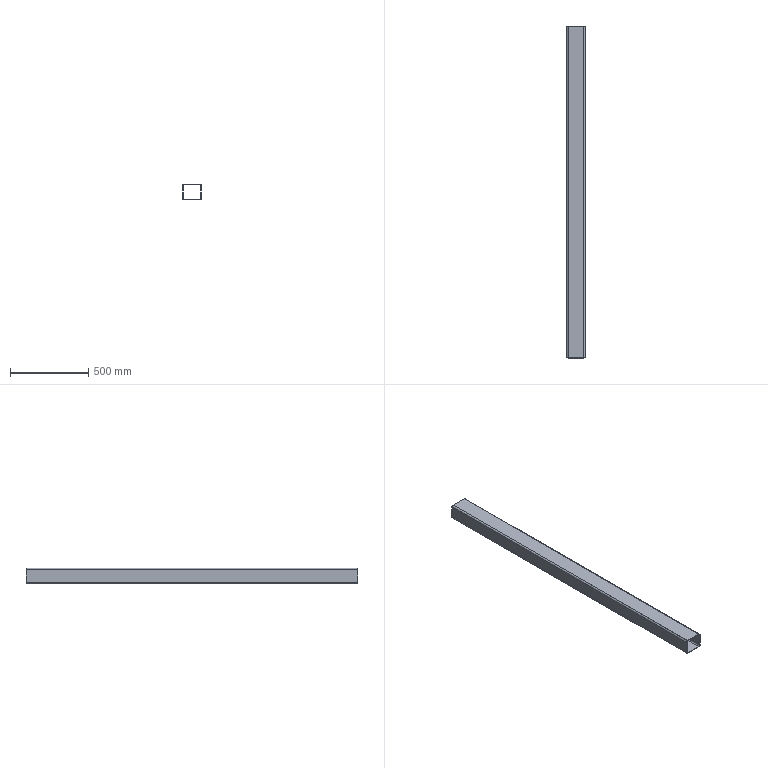Part | SolidWorks | features ExtruThin 1 | 1 solid | 18 faces | box 120 x 2124 x 100 mm | volume 2634230 mm3 | plane 10 | cylinder 8 | commonest cylinder face diameters 14 x4 20 x4
STEP:
#1=CARTESIAN_POINT('',(60.,1062.,-40.));
#2=VERTEX_POINT('',#1);
#3=CARTESIAN_POINT('',(50.,1062.,-50.));
#4=VERTEX_POINT('',#3);
#5=CARTESIAN_POINT('',(50.,1062.,-40.));
#6=DIRECTION('',(0.,1.,0.));
#7=DIRECTION('',(0.,0.,-1.));
#8=AXIS2_PLACEMENT_3D('',#5,#6,#7);
#9=CIRCLE('',#8,10.);
#10=EDGE_CURVE('',#2,#4,#9,.T.);
#11=ORIENTED_EDGE('',*,*,#10,.T.);
#12=CARTESIAN_POINT('',(-50.,1062.,-50.));
#13=VERTEX_POINT('',#12);
#14=CARTESIAN_POINT('',(-50.,1062.,-50.));
#15=DIRECTION('',(-1.,0.,0.));
#16=VECTOR('',#15,1000.);
#17=LINE('',#14,#16);
#18=EDGE_CURVE('',#4,#13,#17,.T.);
#19=ORIENTED_EDGE('',*,*,#18,.T.);
#20=CARTESIAN_POINT('',(-60.,1062.,-40.));
#21=VERTEX_POINT('',#20);
#22=CARTESIAN_POINT('',(-50.,1062.,-40.));
#23=DIRECTION('',(0.,1.,0.));
#24=DIRECTION('',(0.,0.,1.));
#25=AXIS2_PLACEMENT_3D('',#22,#23,#24);
#26=CIRCLE('',#25,10.);
#27=EDGE_CURVE('',#13,#21,#26,.T.);
#28=ORIENTED_EDGE('',*,*,#27,.T.);
#29=CARTESIAN_POINT('',(-60.,1062.,40.));
#30=VERTEX_POINT('',#29);
#31=CARTESIAN_POINT('',(-60.,1062.,-40.));
#32=DIRECTION('',(0.,0.,1.));
#33=VECTOR('',#32,1000.);
#34=LINE('',#31,#33);
#35=EDGE_CURVE('',#21,#30,#34,.T.);
#36=ORIENTED_EDGE('',*,*,#35,.T.);
#37=CARTESIAN_POINT('',(-50.,1062.,50.));
#38=VERTEX_POINT('',#37);
#39=CARTESIAN_POINT('',(-50.,1062.,40.));
#40=DIRECTION('',(0.,1.,0.));
#41=DIRECTION('',(0.,0.,1.));
#42=AXIS2_PLACEMENT_3D('',#39,#40,#41);
#43=CIRCLE('',#42,10.);
#44=EDGE_CURVE('',#30,#38,#43,.T.);
#45=ORIENTED_EDGE('',*,*,#44,.T.);
#46=CARTESIAN_POINT('',(50.,1062.,50.));
#47=VERTEX_POINT('',#46);
#48=CARTESIAN_POINT('',(-50.,1062.,50.));
#49=DIRECTION('',(1.,0.,0.));
#50=VECTOR('',#49,1000.);
#51=LINE('',#48,#50);
#52=EDGE_CURVE('',#38,#47,#51,.T.);
#53=ORIENTED_EDGE('',*,*,#52,.T.);
#54=CARTESIAN_POINT('',(60.,1062.,40.));
#55=VERTEX_POINT('',#54);
#56=CARTESIAN_POINT('',(50.,1062.,40.));
#57=DIRECTION('',(0.,1.,0.));
#58=DIRECTION('',(0.,0.,1.));
#59=AXIS2_PLACEMENT_3D('',#56,#57,#58);
#60=CIRCLE('',#59,10.);
#61=EDGE_CURVE('',#47,#55,#60,.T.);
#62=ORIENTED_EDGE('',*,*,#61,.T.);
#63=CARTESIAN_POINT('',(60.,1062.,-40.));
#64=DIRECTION('',(0.,0.,-1.));
#65=VECTOR('',#64,1000.);
#66=LINE('',#63,#65);
#67=EDGE_CURVE('',#55,#2,#66,.T.);
#68=ORIENTED_EDGE('',*,*,#67,.T.);
#69=EDGE_LOOP('',(#11,#19,#28,#36,#45,#53,#62,#68));
#70=FACE_OUTER_BOUND('',#69,.T.);
#71=CARTESIAN_POINT('',(50.,1062.,-47.));
#72=VERTEX_POINT('',#71);
#73=CARTESIAN_POINT('',(-50.,1062.,-47.));
#74=VERTEX_POINT('',#73);
#75=CARTESIAN_POINT('',(50.,1062.,-47.));
#76=DIRECTION('',(-1.,0.,0.));
#77=VECTOR('',#76,1000.);
#78=LINE('',#75,#77);
#79=EDGE_CURVE('',#72,#74,#78,.T.);
#80=ORIENTED_EDGE('',*,*,#79,.F.);
#81=CARTESIAN_POINT('',(57.,1062.,-40.));
#82=VERTEX_POINT('',#81);
#83=CARTESIAN_POINT('',(50.,1062.,-40.));
#84=DIRECTION('',(0.,1.,0.));
#85=DIRECTION('',(-1.,0.,0.));
#86=AXIS2_PLACEMENT_3D('',#83,#84,#85);
#87=CIRCLE('',#86,7.);
#88=EDGE_CURVE('',#82,#72,#87,.T.);
#89=ORIENTED_EDGE('',*,*,#88,.F.);
#90=CARTESIAN_POINT('',(57.,1062.,40.));
#91=VERTEX_POINT('',#90);
#92=CARTESIAN_POINT('',(57.,1062.,-40.));
#93=DIRECTION('',(0.,0.,-1.));
#94=VECTOR('',#93,1000.);
#95=LINE('',#92,#94);
#96=EDGE_CURVE('',#91,#82,#95,.T.);
#97=ORIENTED_EDGE('',*,*,#96,.F.);
#98=CARTESIAN_POINT('',(50.,1062.,47.));
#99=VERTEX_POINT('',#98);
#100=CARTESIAN_POINT('',(50.,1062.,40.));
#101=DIRECTION('',(0.,1.,0.));
#102=DIRECTION('',(-1.,0.,0.));
#103=AXIS2_PLACEMENT_3D('',#100,#101,#102);
#104=CIRCLE('',#103,7.);
#105=EDGE_CURVE('',#99,#91,#104,.T.);
#106=ORIENTED_EDGE('',*,*,#105,.F.);
#107=CARTESIAN_POINT('',(-50.,1062.,47.));
#108=VERTEX_POINT('',#107);
#109=CARTESIAN_POINT('',(50.,1062.,47.));
#110=DIRECTION('',(1.,0.,0.));
#111=VECTOR('',#110,1000.);
#112=LINE('',#109,#111);
#113=EDGE_CURVE('',#108,#99,#112,.T.);
#114=ORIENTED_EDGE('',*,*,#113,.F.);
#115=CARTESIAN_POINT('',(-57.,1062.,40.));
#116=VERTEX_POINT('',#115);
#117=CARTESIAN_POINT('',(-50.,1062.,40.));
#118=DIRECTION('',(0.,1.,0.));
#119=DIRECTION('',(-1.,0.,0.));
#120=AXIS2_PLACEMENT_3D('',#117,#118,#119);
#121=CIRCLE('',#120,7.);
#122=EDGE_CURVE('',#116,#108,#121,.T.);
#123=ORIENTED_EDGE('',*,*,#122,.F.);
#124=CARTESIAN_POINT('',(-57.,1062.,-40.));
#125=VERTEX_POINT('',#124);
#126=CARTESIAN_POINT('',(-57.,1062.,-40.));
#127=DIRECTION('',(0.,0.,1.));
#128=VECTOR('',#127,1000.);
#129=LINE('',#126,#128);
#130=EDGE_CURVE('',#125,#116,#129,.T.);
#131=ORIENTED_EDGE('',*,*,#130,.F.);
#132=CARTESIAN_POINT('',(-50.,1062.,-40.));
#133=DIRECTION('',(0.,1.,0.));
#134=DIRECTION('',(-1.,0.,0.));
#135=AXIS2_PLACEMENT_3D('',#132,#133,#134);
#136=CIRCLE('',#135,7.);
#137=EDGE_CURVE('',#74,#125,#136,.T.);
#138=ORIENTED_EDGE('',*,*,#137,.F.);
#139=EDGE_LOOP('',(#80,#89,#97,#106,#114,#123,#131,#138));
#140=FACE_BOUND('',#139,.T.);
#141=CARTESIAN_POINT('',(50.,1062.,-40.));
#142=DIRECTION('',(0.,1.,0.));
#143=DIRECTION('',(0.,0.,1.));
#144=AXIS2_PLACEMENT_3D('',#141,#142,#143);
#145=PLANE('',#144);
#146=ADVANCED_FACE('',(#70,#140),#145,.T.);
#147=CARTESIAN_POINT('',(60.,-1062.,-40.));
#148=VERTEX_POINT('',#147);
#149=CARTESIAN_POINT('',(50.,-1062.,-50.));
#150=VERTEX_POINT('',#149);
#151=CARTESIAN_POINT('',(50.,-1062.,-40.));
#152=DIRECTION('',(0.,1.,0.));
#153=DIRECTION('',(0.,0.,-1.));
#154=AXIS2_PLACEMENT_3D('',#151,#152,#153);
#155=CIRCLE('',#154,10.);
#156=EDGE_CURVE('',#148,#150,#155,.T.);
#157=ORIENTED_EDGE('',*,*,#156,.F.);
#158=CARTESIAN_POINT('',(60.,-1062.,40.));
#159=VERTEX_POINT('',#158);
#160=CARTESIAN_POINT('',(60.,-1062.,-40.));
#161=DIRECTION('',(0.,0.,-1.));
#162=VECTOR('',#161,1000.);
#163=LINE('',#160,#162);
#164=EDGE_CURVE('',#159,#148,#163,.T.);
#165=ORIENTED_EDGE('',*,*,#164,.F.);
#166=CARTESIAN_POINT('',(50.,-1062.,50.));
#167=VERTEX_POINT('',#166);
#168=CARTESIAN_POINT('',(50.,-1062.,40.));
#169=DIRECTION('',(0.,1.,0.));
#170=DIRECTION('',(0.,0.,1.));
#171=AXIS2_PLACEMENT_3D('',#168,#169,#170);
#172=CIRCLE('',#171,10.);
#173=EDGE_CURVE('',#167,#159,#172,.T.);
#174=ORIENTED_EDGE('',*,*,#173,.F.);
#175=CARTESIAN_POINT('',(-50.,-1062.,50.));
#176=VERTEX_POINT('',#175);
#177=CARTESIAN_POINT('',(-50.,-1062.,50.));
#178=DIRECTION('',(1.,0.,0.));
#179=VECTOR('',#178,1000.);
#180=LINE('',#177,#179);
#181=EDGE_CURVE('',#176,#167,#180,.T.);
#182=ORIENTED_EDGE('',*,*,#181,.F.);
#183=CARTESIAN_POINT('',(-60.,-1062.,40.));
#184=VERTEX_POINT('',#183);
#185=CARTESIAN_POINT('',(-50.,-1062.,40.));
#186=DIRECTION('',(0.,1.,0.));
#187=DIRECTION('',(0.,0.,1.));
#188=AXIS2_PLACEMENT_3D('',#185,#186,#187);
#189=CIRCLE('',#188,10.);
#190=EDGE_CURVE('',#184,#176,#189,.T.);
#191=ORIENTED_EDGE('',*,*,#190,.F.);
#192=CARTESIAN_POINT('',(-60.,-1062.,-40.));
#193=VERTEX_POINT('',#192);
#194=CARTESIAN_POINT('',(-60.,-1062.,-40.));
#195=DIRECTION('',(0.,0.,1.));
#196=VECTOR('',#195,1000.);
#197=LINE('',#194,#196);
#198=EDGE_CURVE('',#193,#184,#197,.T.);
#199=ORIENTED_EDGE('',*,*,#198,.F.);
#200=CARTESIAN_POINT('',(-50.,-1062.,-50.));
#201=VERTEX_POINT('',#200);
#202=CARTESIAN_POINT('',(-50.,-1062.,-40.));
#203=DIRECTION('',(0.,1.,0.));
#204=DIRECTION('',(0.,0.,1.));
#205=AXIS2_PLACEMENT_3D('',#202,#203,#204);
#206=CIRCLE('',#205,10.);
#207=EDGE_CURVE('',#201,#193,#206,.T.);
#208=ORIENTED_EDGE('',*,*,#207,.F.);
#209=CARTESIAN_POINT('',(-50.,-1062.,-50.));
#210=DIRECTION('',(-1.,0.,0.));
#211=VECTOR('',#210,1000.);
#212=LINE('',#209,#211);
#213=EDGE_CURVE('',#150,#201,#212,.T.);
#214=ORIENTED_EDGE('',*,*,#213,.F.);
#215=EDGE_LOOP('',(#157,#165,#174,#182,#191,#199,#208,#214));
#216=FACE_OUTER_BOUND('',#215,.T.);
#217=CARTESIAN_POINT('',(57.,-1062.,-40.));
#218=VERTEX_POINT('',#217);
#219=CARTESIAN_POINT('',(50.,-1062.,-47.));
#220=VERTEX_POINT('',#219);
#221=CARTESIAN_POINT('',(50.,-1062.,-40.));
#222=DIRECTION('',(0.,1.,0.));
#223=DIRECTION('',(-1.,0.,0.));
#224=AXIS2_PLACEMENT_3D('',#221,#222,#223);
#225=CIRCLE('',#224,7.);
#226=EDGE_CURVE('',#218,#220,#225,.T.);
#227=ORIENTED_EDGE('',*,*,#226,.T.);
#228=CARTESIAN_POINT('',(-50.,-1062.,-47.));
#229=VERTEX_POINT('',#228);
#230=CARTESIAN_POINT('',(50.,-1062.,-47.));
#231=DIRECTION('',(-1.,0.,0.));
#232=VECTOR('',#231,1000.);
#233=LINE('',#230,#232);
#234=EDGE_CURVE('',#220,#229,#233,.T.);
#235=ORIENTED_EDGE('',*,*,#234,.T.);
#236=CARTESIAN_POINT('',(-57.,-1062.,-40.));
#237=VERTEX_POINT('',#236);
#238=CARTESIAN_POINT('',(-50.,-1062.,-40.));
#239=DIRECTION('',(0.,1.,0.));
#240=DIRECTION('',(-1.,0.,0.));
#241=AXIS2_PLACEMENT_3D('',#238,#239,#240);
#242=CIRCLE('',#241,7.);
#243=EDGE_CURVE('',#229,#237,#242,.T.);
#244=ORIENTED_EDGE('',*,*,#243,.T.);
#245=CARTESIAN_POINT('',(-57.,-1062.,40.));
#246=VERTEX_POINT('',#245);
#247=CARTESIAN_POINT('',(-57.,-1062.,-40.));
#248=DIRECTION('',(0.,0.,1.));
#249=VECTOR('',#248,1000.);
#250=LINE('',#247,#249);
#251=EDGE_CURVE('',#237,#246,#250,.T.);
#252=ORIENTED_EDGE('',*,*,#251,.T.);
#253=CARTESIAN_POINT('',(-50.,-1062.,47.));
#254=VERTEX_POINT('',#253);
#255=CARTESIAN_POINT('',(-50.,-1062.,40.));
#256=DIRECTION('',(0.,1.,0.));
#257=DIRECTION('',(-1.,0.,0.));
#258=AXIS2_PLACEMENT_3D('',#255,#256,#257);
#259=CIRCLE('',#258,7.);
#260=EDGE_CURVE('',#246,#254,#259,.T.);
#261=ORIENTED_EDGE('',*,*,#260,.T.);
#262=CARTESIAN_POINT('',(50.,-1062.,47.));
#263=VERTEX_POINT('',#262);
#264=CARTESIAN_POINT('',(50.,-1062.,47.));
#265=DIRECTION('',(1.,0.,0.));
#266=VECTOR('',#265,1000.);
#267=LINE('',#264,#266);
#268=EDGE_CURVE('',#254,#263,#267,.T.);
#269=ORIENTED_EDGE('',*,*,#268,.T.);
#270=CARTESIAN_POINT('',(57.,-1062.,40.));
#271=VERTEX_POINT('',#270);
#272=CARTESIAN_POINT('',(50.,-1062.,40.));
#273=DIRECTION('',(0.,1.,0.));
#274=DIRECTION('',(-1.,0.,0.));
#275=AXIS2_PLACEMENT_3D('',#272,#273,#274);
#276=CIRCLE('',#275,7.);
#277=EDGE_CURVE('',#263,#271,#276,.T.);
#278=ORIENTED_EDGE('',*,*,#277,.T.);
#279=CARTESIAN_POINT('',(57.,-1062.,-40.));
#280=DIRECTION('',(0.,0.,-1.));
#281=VECTOR('',#280,1000.);
#282=LINE('',#279,#281);
#283=EDGE_CURVE('',#271,#218,#282,.T.);
#284=ORIENTED_EDGE('',*,*,#283,.T.);
#285=EDGE_LOOP('',(#227,#235,#244,#252,#261,#269,#278,#284));
#286=FACE_BOUND('',#285,.T.);
#287=CARTESIAN_POINT('',(50.,-1062.,-40.));
#288=DIRECTION('',(0.,1.,0.));
#289=DIRECTION('',(0.,0.,1.));
#290=AXIS2_PLACEMENT_3D('',#287,#288,#289);
#291=PLANE('',#290);
#292=ADVANCED_FACE('',(#216,#286),#291,.F.);
#293=ORIENTED_EDGE('',*,*,#156,.T.);
#294=CARTESIAN_POINT('',(50.,1062.,-50.));
#295=DIRECTION('',(0.,-1.,0.));
#296=VECTOR('',#295,1000.);
#297=LINE('',#294,#296);
#298=EDGE_CURVE('',#4,#150,#297,.T.);
#299=ORIENTED_EDGE('',*,*,#298,.F.);
#300=ORIENTED_EDGE('',*,*,#10,.F.);
#301=CARTESIAN_POINT('',(60.,1062.,-40.));
#302=DIRECTION('',(0.,-1.,0.));
#303=VECTOR('',#302,1000.);
#304=LINE('',#301,#303);
#305=EDGE_CURVE('',#2,#148,#304,.T.);
#306=ORIENTED_EDGE('',*,*,#305,.T.);
#307=EDGE_LOOP('',(#293,#299,#300,#306));
#308=FACE_OUTER_BOUND('',#307,.T.);
#309=CARTESIAN_POINT('',(50.,1062.,-40.));
#310=DIRECTION('',(0.,-1.,0.));
#311=DIRECTION('',(0.,0.,-1.));
#312=AXIS2_PLACEMENT_3D('',#309,#310,#311);
#313=CYLINDRICAL_SURFACE('',#312,10.);
#314=ADVANCED_FACE('',(#308),#313,.T.);
#315=ORIENTED_EDGE('',*,*,#213,.T.);
#316=CARTESIAN_POINT('',(-50.,1062.,-50.));
#317=DIRECTION('',(0.,-1.,0.));
#318=VECTOR('',#317,1000.);
#319=LINE('',#316,#318);
#320=EDGE_CURVE('',#13,#201,#319,.T.);
#321=ORIENTED_EDGE('',*,*,#320,.F.);
#322=ORIENTED_EDGE('',*,*,#18,.F.);
#323=ORIENTED_EDGE('',*,*,#298,.T.);
#324=EDGE_LOOP('',(#315,#321,#322,#323));
#325=FACE_OUTER_BOUND('',#324,.T.);
#326=CARTESIAN_POINT('',(-50.,1062.,-50.));
#327=DIRECTION('',(0.,0.,1.));
#328=DIRECTION('',(1.,0.,0.));
#329=AXIS2_PLACEMENT_3D('',#326,#327,#328);
#330=PLANE('',#329);
#331=ADVANCED_FACE('',(#325),#330,.F.);
#332=ORIENTED_EDGE('',*,*,#207,.T.);
#333=CARTESIAN_POINT('',(-60.,1062.,-40.));
#334=DIRECTION('',(0.,-1.,0.));
#335=VECTOR('',#334,1000.);
#336=LINE('',#333,#335);
#337=EDGE_CURVE('',#21,#193,#336,.T.);
#338=ORIENTED_EDGE('',*,*,#337,.F.);
#339=ORIENTED_EDGE('',*,*,#27,.F.);
#340=ORIENTED_EDGE('',*,*,#320,.T.);
#341=EDGE_LOOP('',(#332,#338,#339,#340));
#342=FACE_OUTER_BOUND('',#341,.T.);
#343=CARTESIAN_POINT('',(-50.,1062.,-40.));
#344=DIRECTION('',(0.,-1.,0.));
#345=DIRECTION('',(0.,0.,-1.));
#346=AXIS2_PLACEMENT_3D('',#343,#344,#345);
#347=CYLINDRICAL_SURFACE('',#346,10.);
#348=ADVANCED_FACE('',(#342),#347,.T.);
#349=ORIENTED_EDGE('',*,*,#198,.T.);
#350=CARTESIAN_POINT('',(-60.,1062.,40.));
#351=DIRECTION('',(0.,-1.,0.));
#352=VECTOR('',#351,1000.);
#353=LINE('',#350,#352);
#354=EDGE_CURVE('',#30,#184,#353,.T.);
#355=ORIENTED_EDGE('',*,*,#354,.F.);
#356=ORIENTED_EDGE('',*,*,#35,.F.);
#357=ORIENTED_EDGE('',*,*,#337,.T.);
#358=EDGE_LOOP('',(#349,#355,#356,#357));
#359=FACE_OUTER_BOUND('',#358,.T.);
#360=CARTESIAN_POINT('',(-60.,1062.,-40.));
#361=DIRECTION('',(1.,0.,0.));
#362=DIRECTION('',(0.,0.,-1.));
#363=AXIS2_PLACEMENT_3D('',#360,#361,#362);
#364=PLANE('',#363);
#365=ADVANCED_FACE('',(#359),#364,.F.);
#366=ORIENTED_EDGE('',*,*,#190,.T.);
#367=CARTESIAN_POINT('',(-50.,1062.,50.));
#368=DIRECTION('',(0.,-1.,0.));
#369=VECTOR('',#368,1000.);
#370=LINE('',#367,#369);
#371=EDGE_CURVE('',#38,#176,#370,.T.);
#372=ORIENTED_EDGE('',*,*,#371,.F.);
#373=ORIENTED_EDGE('',*,*,#44,.F.);
#374=ORIENTED_EDGE('',*,*,#354,.T.);
#375=EDGE_LOOP('',(#366,#372,#373,#374));
#376=FACE_OUTER_BOUND('',#375,.T.);
#377=CARTESIAN_POINT('',(-50.,1062.,40.));
#378=DIRECTION('',(0.,-1.,0.));
#379=DIRECTION('',(0.,0.,-1.));
#380=AXIS2_PLACEMENT_3D('',#377,#378,#379);
#381=CYLINDRICAL_SURFACE('',#380,10.);
#382=ADVANCED_FACE('',(#376),#381,.T.);
#383=ORIENTED_EDGE('',*,*,#181,.T.);
#384=CARTESIAN_POINT('',(50.,1062.,50.));
#385=DIRECTION('',(0.,-1.,0.));
#386=VECTOR('',#385,1000.);
#387=LINE('',#384,#386);
#388=EDGE_CURVE('',#47,#167,#387,.T.);
#389=ORIENTED_EDGE('',*,*,#388,.F.);
#390=ORIENTED_EDGE('',*,*,#52,.F.);
#391=ORIENTED_EDGE('',*,*,#371,.T.);
#392=EDGE_LOOP('',(#383,#389,#390,#391));
#393=FACE_OUTER_BOUND('',#392,.T.);
#394=CARTESIAN_POINT('',(-50.,1062.,50.));
#395=DIRECTION('',(0.,0.,-1.));
#396=DIRECTION('',(-1.,0.,0.));
#397=AXIS2_PLACEMENT_3D('',#394,#395,#396);
#398=PLANE('',#397);
#399=ADVANCED_FACE('',(#393),#398,.F.);
#400=ORIENTED_EDGE('',*,*,#173,.T.);
#401=CARTESIAN_POINT('',(60.,1062.,40.));
#402=DIRECTION('',(0.,-1.,0.));
#403=VECTOR('',#402,1000.);
#404=LINE('',#401,#403);
#405=EDGE_CURVE('',#55,#159,#404,.T.);
#406=ORIENTED_EDGE('',*,*,#405,.F.);
#407=ORIENTED_EDGE('',*,*,#61,.F.);
#408=ORIENTED_EDGE('',*,*,#388,.T.);
#409=EDGE_LOOP('',(#400,#406,#407,#408));
#410=FACE_OUTER_BOUND('',#409,.T.);
#411=CARTESIAN_POINT('',(50.,1062.,40.));
#412=DIRECTION('',(0.,-1.,0.));
#413=DIRECTION('',(0.,0.,-1.));
#414=AXIS2_PLACEMENT_3D('',#411,#412,#413);
#415=CYLINDRICAL_SURFACE('',#414,10.);
#416=ADVANCED_FACE('',(#410),#415,.T.);
#417=ORIENTED_EDGE('',*,*,#164,.T.);
#418=ORIENTED_EDGE('',*,*,#305,.F.);
#419=ORIENTED_EDGE('',*,*,#67,.F.);
#420=ORIENTED_EDGE('',*,*,#405,.T.);
#421=EDGE_LOOP('',(#417,#418,#419,#420));
#422=FACE_OUTER_BOUND('',#421,.T.);
#423=CARTESIAN_POINT('',(60.,1062.,-40.));
#424=DIRECTION('',(-1.,0.,0.));
#425=DIRECTION('',(0.,0.,1.));
#426=AXIS2_PLACEMENT_3D('',#423,#424,#425);
#427=PLANE('',#426);
#428=ADVANCED_FACE('',(#422),#427,.F.);
#429=ORIENTED_EDGE('',*,*,#226,.F.);
#430=CARTESIAN_POINT('',(57.,1062.,-40.));
#431=DIRECTION('',(0.,-1.,0.));
#432=VECTOR('',#431,1000.);
#433=LINE('',#430,#432);
#434=EDGE_CURVE('',#82,#218,#433,.T.);
#435=ORIENTED_EDGE('',*,*,#434,.F.);
#436=ORIENTED_EDGE('',*,*,#88,.T.);
#437=CARTESIAN_POINT('',(50.,1062.,-47.));
#438=DIRECTION('',(0.,-1.,0.));
#439=VECTOR('',#438,1000.);
#440=LINE('',#437,#439);
#441=EDGE_CURVE('',#72,#220,#440,.T.);
#442=ORIENTED_EDGE('',*,*,#441,.T.);
#443=EDGE_LOOP('',(#429,#435,#436,#442));
#444=FACE_OUTER_BOUND('',#443,.T.);
#445=CARTESIAN_POINT('',(50.,1062.,-40.));
#446=DIRECTION('',(0.,-1.,0.));
#447=DIRECTION('',(0.,0.,-1.));
#448=AXIS2_PLACEMENT_3D('',#445,#446,#447);
#449=CYLINDRICAL_SURFACE('',#448,7.);
#450=ADVANCED_FACE('',(#444),#449,.F.);
#451=ORIENTED_EDGE('',*,*,#234,.F.);
#452=ORIENTED_EDGE('',*,*,#441,.F.);
#453=ORIENTED_EDGE('',*,*,#79,.T.);
#454=CARTESIAN_POINT('',(-50.,1062.,-47.));
#455=DIRECTION('',(0.,-1.,0.));
#456=VECTOR('',#455,1000.);
#457=LINE('',#454,#456);
#458=EDGE_CURVE('',#74,#229,#457,.T.);
#459=ORIENTED_EDGE('',*,*,#458,.T.);
#460=EDGE_LOOP('',(#451,#452,#453,#459));
#461=FACE_OUTER_BOUND('',#460,.T.);
#462=CARTESIAN_POINT('',(50.,1062.,-47.));
#463=DIRECTION('',(0.,0.,1.));
#464=DIRECTION('',(1.,0.,0.));
#465=AXIS2_PLACEMENT_3D('',#462,#463,#464);
#466=PLANE('',#465);
#467=ADVANCED_FACE('',(#461),#466,.T.);
#468=ORIENTED_EDGE('',*,*,#243,.F.);
#469=ORIENTED_EDGE('',*,*,#458,.F.);
#470=ORIENTED_EDGE('',*,*,#137,.T.);
#471=CARTESIAN_POINT('',(-57.,1062.,-40.));
#472=DIRECTION('',(0.,-1.,0.));
#473=VECTOR('',#472,1000.);
#474=LINE('',#471,#473);
#475=EDGE_CURVE('',#125,#237,#474,.T.);
#476=ORIENTED_EDGE('',*,*,#475,.T.);
#477=EDGE_LOOP('',(#468,#469,#470,#476));
#478=FACE_OUTER_BOUND('',#477,.T.);
#479=CARTESIAN_POINT('',(-50.,1062.,-40.));
#480=DIRECTION('',(0.,-1.,0.));
#481=DIRECTION('',(0.,0.,-1.));
#482=AXIS2_PLACEMENT_3D('',#479,#480,#481);
#483=CYLINDRICAL_SURFACE('',#482,7.);
#484=ADVANCED_FACE('',(#478),#483,.F.);
#485=ORIENTED_EDGE('',*,*,#251,.F.);
#486=ORIENTED_EDGE('',*,*,#475,.F.);
#487=ORIENTED_EDGE('',*,*,#130,.T.);
#488=CARTESIAN_POINT('',(-57.,1062.,40.));
#489=DIRECTION('',(0.,-1.,0.));
#490=VECTOR('',#489,1000.);
#491=LINE('',#488,#490);
#492=EDGE_CURVE('',#116,#246,#491,.T.);
#493=ORIENTED_EDGE('',*,*,#492,.T.);
#494=EDGE_LOOP('',(#485,#486,#487,#493));
#495=FACE_OUTER_BOUND('',#494,.T.);
#496=CARTESIAN_POINT('',(-57.,1062.,-40.));
#497=DIRECTION('',(1.,0.,0.));
#498=DIRECTION('',(0.,0.,-1.));
#499=AXIS2_PLACEMENT_3D('',#496,#497,#498);
#500=PLANE('',#499);
#501=ADVANCED_FACE('',(#495),#500,.T.);
#502=ORIENTED_EDGE('',*,*,#260,.F.);
#503=ORIENTED_EDGE('',*,*,#492,.F.);
#504=ORIENTED_EDGE('',*,*,#122,.T.);
#505=CARTESIAN_POINT('',(-50.,1062.,47.));
#506=DIRECTION('',(0.,-1.,0.));
#507=VECTOR('',#506,1000.);
#508=LINE('',#505,#507);
#509=EDGE_CURVE('',#108,#254,#508,.T.);
#510=ORIENTED_EDGE('',*,*,#509,.T.);
#511=EDGE_LOOP('',(#502,#503,#504,#510));
#512=FACE_OUTER_BOUND('',#511,.T.);
#513=CARTESIAN_POINT('',(-50.,1062.,40.));
#514=DIRECTION('',(0.,-1.,0.));
#515=DIRECTION('',(0.,0.,-1.));
#516=AXIS2_PLACEMENT_3D('',#513,#514,#515);
#517=CYLINDRICAL_SURFACE('',#516,7.);
#518=ADVANCED_FACE('',(#512),#517,.F.);
#519=ORIENTED_EDGE('',*,*,#268,.F.);
#520=ORIENTED_EDGE('',*,*,#509,.F.);
#521=ORIENTED_EDGE('',*,*,#113,.T.);
#522=CARTESIAN_POINT('',(50.,1062.,47.));
#523=DIRECTION('',(0.,-1.,0.));
#524=VECTOR('',#523,1000.);
#525=LINE('',#522,#524);
#526=EDGE_CURVE('',#99,#263,#525,.T.);
#527=ORIENTED_EDGE('',*,*,#526,.T.);
#528=EDGE_LOOP('',(#519,#520,#521,#527));
#529=FACE_OUTER_BOUND('',#528,.T.);
#530=CARTESIAN_POINT('',(50.,1062.,47.));
#531=DIRECTION('',(0.,0.,-1.));
#532=DIRECTION('',(-1.,0.,0.));
#533=AXIS2_PLACEMENT_3D('',#530,#531,#532);
#534=PLANE('',#533);
#535=ADVANCED_FACE('',(#529),#534,.T.);
#536=ORIENTED_EDGE('',*,*,#277,.F.);
#537=ORIENTED_EDGE('',*,*,#526,.F.);
#538=ORIENTED_EDGE('',*,*,#105,.T.);
#539=CARTESIAN_POINT('',(57.,1062.,40.));
#540=DIRECTION('',(0.,-1.,0.));
#541=VECTOR('',#540,1000.);
#542=LINE('',#539,#541);
#543=EDGE_CURVE('',#91,#271,#542,.T.);
#544=ORIENTED_EDGE('',*,*,#543,.T.);
#545=EDGE_LOOP('',(#536,#537,#538,#544));
#546=FACE_OUTER_BOUND('',#545,.T.);
#547=CARTESIAN_POINT('',(50.,1062.,40.));
#548=DIRECTION('',(0.,-1.,0.));
#549=DIRECTION('',(0.,0.,-1.));
#550=AXIS2_PLACEMENT_3D('',#547,#548,#549);
#551=CYLINDRICAL_SURFACE('',#550,7.);
#552=ADVANCED_FACE('',(#546),#551,.F.);
#553=ORIENTED_EDGE('',*,*,#283,.F.);
#554=ORIENTED_EDGE('',*,*,#543,.F.);
#555=ORIENTED_EDGE('',*,*,#96,.T.);
#556=ORIENTED_EDGE('',*,*,#434,.T.);
#557=EDGE_LOOP('',(#553,#554,#555,#556));
#558=FACE_OUTER_BOUND('',#557,.T.);
#559=CARTESIAN_POINT('',(57.,1062.,-40.));
#560=DIRECTION('',(-1.,0.,0.));
#561=DIRECTION('',(0.,0.,1.));
#562=AXIS2_PLACEMENT_3D('',#559,#560,#561);
#563=PLANE('',#562);
#564=ADVANCED_FACE('',(#558),#563,.T.);
#565=CLOSED_SHELL('',(#146,#292,#314,#331,#348,#365,#382,#399,#416,#428,#450,#467,#484,#501,#518,#535,#552,#564));
#566=MANIFOLD_SOLID_BREP('',#565);
#567=CARTESIAN_POINT('',(0.,0.,0.));
#568=DIRECTION('',(0.,0.,1.));
#569=DIRECTION('',(1.,0.,0.));
#570=AXIS2_PLACEMENT_3D('',#567,#568,#569);
#571=(LENGTH_UNIT()NAMED_UNIT(*)SI_UNIT(.MILLI.,.METRE.));
#572=UNCERTAINTY_MEASURE_WITH_UNIT(LENGTH_MEASURE(0.00001),#571,'','');
#573=(NAMED_UNIT(*)PLANE_ANGLE_UNIT()SI_UNIT($,.RADIAN.));
#574=(NAMED_UNIT(*)SI_UNIT($,.STERADIAN.)SOLID_ANGLE_UNIT());
#575=(GEOMETRIC_REPRESENTATION_CONTEXT(3)GLOBAL_UNCERTAINTY_ASSIGNED_CONTEXT((#572))GLOBAL_UNIT_ASSIGNED_CONTEXT((#571,#573,#574))REPRESENTATION_CONTEXT('',''));
#576=ADVANCED_BREP_SHAPE_REPRESENTATION('',(#566,#570),#575);